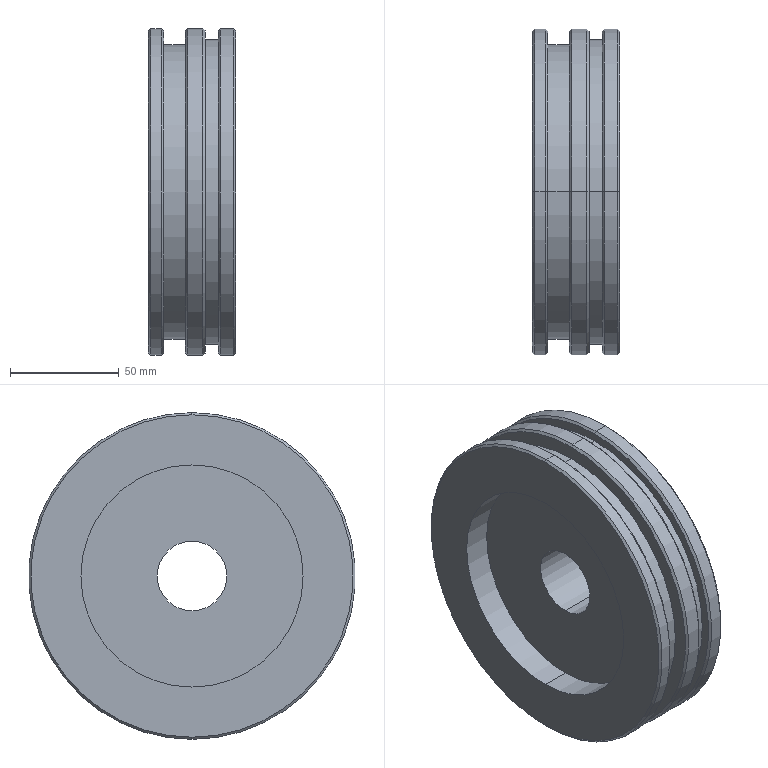Part | SolidWorks | features Chamfer 1, Revolution 1 | 1 solid | 39 faces | box 40 x 150 x 150 mm | volume 516029 mm3 | cone 16 | cylinder 14 | plane 9 | commonest cylinder face diameters 150 x6 32 x2 102 x2 135 x2 140 x2
STEP:
#1=CARTESIAN_POINT('',(0.,0.,74.));
#2=VERTEX_POINT('',#1);
#3=CARTESIAN_POINT('',(0.,0.,-74.));
#4=VERTEX_POINT('',#3);
#5=CARTESIAN_POINT('',(0.,0.,0.));
#6=DIRECTION('',(-1.,0.,0.));
#7=DIRECTION('',(0.,0.,-1.));
#8=AXIS2_PLACEMENT_3D('',#5,#6,#7);
#9=CIRCLE('',#8,74.);
#10=EDGE_CURVE('',#2,#4,#9,.T.);
#11=ORIENTED_EDGE('',*,*,#10,.F.);
#12=CARTESIAN_POINT('',(1.,0.,75.));
#13=VERTEX_POINT('',#12);
#14=CARTESIAN_POINT('',(0.,0.,74.));
#15=DIRECTION('',(0.7071,0.,0.7071));
#16=VECTOR('',#15,1000.);
#17=LINE('',#14,#16);
#18=EDGE_CURVE('',#2,#13,#17,.T.);
#19=ORIENTED_EDGE('',*,*,#18,.T.);
#20=CARTESIAN_POINT('',(1.,0.,-75.));
#21=VERTEX_POINT('',#20);
#22=CARTESIAN_POINT('',(1.,0.,0.));
#23=DIRECTION('',(1.,0.,0.));
#24=DIRECTION('',(0.,0.,-1.));
#25=AXIS2_PLACEMENT_3D('',#22,#23,#24);
#26=CIRCLE('',#25,75.);
#27=EDGE_CURVE('',#21,#13,#26,.T.);
#28=ORIENTED_EDGE('',*,*,#27,.F.);
#29=CARTESIAN_POINT('',(0.,0.,-74.));
#30=DIRECTION('',(0.7071,0.,-0.7071));
#31=VECTOR('',#30,1000.);
#32=LINE('',#29,#31);
#33=EDGE_CURVE('',#4,#21,#32,.T.);
#34=ORIENTED_EDGE('',*,*,#33,.F.);
#35=EDGE_LOOP('',(#11,#19,#28,#34));
#36=FACE_OUTER_BOUND('',#35,.T.);
#37=CARTESIAN_POINT('',(0.,0.,0.));
#38=DIRECTION('',(1.,0.,0.));
#39=DIRECTION('',(0.,0.,-1.));
#40=AXIS2_PLACEMENT_3D('',#37,#38,#39);
#41=CONICAL_SURFACE('',#40,74.,0.7854);
#42=ADVANCED_FACE('',(#36),#41,.T.);
#43=CARTESIAN_POINT('',(7.,0.,-74.));
#44=VERTEX_POINT('',#43);
#45=CARTESIAN_POINT('',(7.,0.,74.));
#46=VERTEX_POINT('',#45);
#47=CARTESIAN_POINT('',(7.,0.,0.));
#48=DIRECTION('',(1.,0.,0.));
#49=DIRECTION('',(0.,0.,1.));
#50=AXIS2_PLACEMENT_3D('',#47,#48,#49);
#51=CIRCLE('',#50,74.);
#52=EDGE_CURVE('',#44,#46,#51,.T.);
#53=ORIENTED_EDGE('',*,*,#52,.F.);
#54=CARTESIAN_POINT('',(6.,0.,-75.));
#55=VERTEX_POINT('',#54);
#56=CARTESIAN_POINT('',(6.,0.,-75.));
#57=DIRECTION('',(-0.7071,0.,-0.7071));
#58=VECTOR('',#57,1000.);
#59=LINE('',#56,#58);
#60=EDGE_CURVE('',#44,#55,#59,.T.);
#61=ORIENTED_EDGE('',*,*,#60,.T.);
#62=CARTESIAN_POINT('',(6.,0.,75.));
#63=VERTEX_POINT('',#62);
#64=CARTESIAN_POINT('',(6.,0.,0.));
#65=DIRECTION('',(-1.,0.,0.));
#66=DIRECTION('',(0.,0.,1.));
#67=AXIS2_PLACEMENT_3D('',#64,#65,#66);
#68=CIRCLE('',#67,75.);
#69=EDGE_CURVE('',#63,#55,#68,.T.);
#70=ORIENTED_EDGE('',*,*,#69,.F.);
#71=CARTESIAN_POINT('',(6.,0.,75.));
#72=DIRECTION('',(-0.7071,0.,0.7071));
#73=VECTOR('',#72,1000.);
#74=LINE('',#71,#73);
#75=EDGE_CURVE('',#46,#63,#74,.T.);
#76=ORIENTED_EDGE('',*,*,#75,.F.);
#77=EDGE_LOOP('',(#53,#61,#70,#76));
#78=FACE_OUTER_BOUND('',#77,.T.);
#79=CARTESIAN_POINT('',(6.,0.,0.));
#80=DIRECTION('',(-1.,0.,0.));
#81=DIRECTION('',(0.,0.,1.));
#82=AXIS2_PLACEMENT_3D('',#79,#80,#81);
#83=CONICAL_SURFACE('',#82,75.,0.7854);
#84=ADVANCED_FACE('',(#78),#83,.T.);
#85=CARTESIAN_POINT('',(17.,0.,74.));
#86=VERTEX_POINT('',#85);
#87=CARTESIAN_POINT('',(17.,0.,-74.));
#88=VERTEX_POINT('',#87);
#89=CARTESIAN_POINT('',(17.,0.,0.));
#90=DIRECTION('',(-1.,0.,0.));
#91=DIRECTION('',(0.,0.,-1.));
#92=AXIS2_PLACEMENT_3D('',#89,#90,#91);
#93=CIRCLE('',#92,74.);
#94=EDGE_CURVE('',#86,#88,#93,.T.);
#95=ORIENTED_EDGE('',*,*,#94,.F.);
#96=CARTESIAN_POINT('',(18.,0.,75.));
#97=VERTEX_POINT('',#96);
#98=CARTESIAN_POINT('',(17.,0.,74.));
#99=DIRECTION('',(0.7071,0.,0.7071));
#100=VECTOR('',#99,1000.);
#101=LINE('',#98,#100);
#102=EDGE_CURVE('',#86,#97,#101,.T.);
#103=ORIENTED_EDGE('',*,*,#102,.T.);
#104=CARTESIAN_POINT('',(18.,0.,-75.));
#105=VERTEX_POINT('',#104);
#106=CARTESIAN_POINT('',(18.,0.,0.));
#107=DIRECTION('',(1.,0.,0.));
#108=DIRECTION('',(0.,0.,-1.));
#109=AXIS2_PLACEMENT_3D('',#106,#107,#108);
#110=CIRCLE('',#109,75.);
#111=EDGE_CURVE('',#105,#97,#110,.T.);
#112=ORIENTED_EDGE('',*,*,#111,.F.);
#113=CARTESIAN_POINT('',(17.,0.,-74.));
#114=DIRECTION('',(0.7071,0.,-0.7071));
#115=VECTOR('',#114,1000.);
#116=LINE('',#113,#115);
#117=EDGE_CURVE('',#88,#105,#116,.T.);
#118=ORIENTED_EDGE('',*,*,#117,.F.);
#119=EDGE_LOOP('',(#95,#103,#112,#118));
#120=FACE_OUTER_BOUND('',#119,.T.);
#121=CARTESIAN_POINT('',(17.,0.,0.));
#122=DIRECTION('',(1.,0.,0.));
#123=DIRECTION('',(0.,0.,-1.));
#124=AXIS2_PLACEMENT_3D('',#121,#122,#123);
#125=CONICAL_SURFACE('',#124,74.,0.7854);
#126=ADVANCED_FACE('',(#120),#125,.T.);
#127=CARTESIAN_POINT('',(26.,0.,-74.));
#128=VERTEX_POINT('',#127);
#129=CARTESIAN_POINT('',(26.,0.,74.));
#130=VERTEX_POINT('',#129);
#131=CARTESIAN_POINT('',(26.,0.,0.));
#132=DIRECTION('',(1.,0.,0.));
#133=DIRECTION('',(0.,0.,1.));
#134=AXIS2_PLACEMENT_3D('',#131,#132,#133);
#135=CIRCLE('',#134,74.);
#136=EDGE_CURVE('',#128,#130,#135,.T.);
#137=ORIENTED_EDGE('',*,*,#136,.F.);
#138=CARTESIAN_POINT('',(25.,0.,-75.));
#139=VERTEX_POINT('',#138);
#140=CARTESIAN_POINT('',(25.,0.,-75.));
#141=DIRECTION('',(-0.7071,0.,-0.7071));
#142=VECTOR('',#141,1000.);
#143=LINE('',#140,#142);
#144=EDGE_CURVE('',#128,#139,#143,.T.);
#145=ORIENTED_EDGE('',*,*,#144,.T.);
#146=CARTESIAN_POINT('',(25.,0.,75.));
#147=VERTEX_POINT('',#146);
#148=CARTESIAN_POINT('',(25.,0.,0.));
#149=DIRECTION('',(-1.,0.,0.));
#150=DIRECTION('',(0.,0.,1.));
#151=AXIS2_PLACEMENT_3D('',#148,#149,#150);
#152=CIRCLE('',#151,75.);
#153=EDGE_CURVE('',#147,#139,#152,.T.);
#154=ORIENTED_EDGE('',*,*,#153,.F.);
#155=CARTESIAN_POINT('',(25.,0.,75.));
#156=DIRECTION('',(-0.7071,0.,0.7071));
#157=VECTOR('',#156,1000.);
#158=LINE('',#155,#157);
#159=EDGE_CURVE('',#130,#147,#158,.T.);
#160=ORIENTED_EDGE('',*,*,#159,.F.);
#161=EDGE_LOOP('',(#137,#145,#154,#160));
#162=FACE_OUTER_BOUND('',#161,.T.);
#163=CARTESIAN_POINT('',(25.,0.,0.));
#164=DIRECTION('',(-1.,0.,0.));
#165=DIRECTION('',(0.,0.,1.));
#166=AXIS2_PLACEMENT_3D('',#163,#164,#165);
#167=CONICAL_SURFACE('',#166,75.,0.7854);
#168=ADVANCED_FACE('',(#162),#167,.T.);
#169=CARTESIAN_POINT('',(32.,0.,74.));
#170=VERTEX_POINT('',#169);
#171=CARTESIAN_POINT('',(32.,0.,-74.));
#172=VERTEX_POINT('',#171);
#173=CARTESIAN_POINT('',(32.,0.,0.));
#174=DIRECTION('',(-1.,0.,0.));
#175=DIRECTION('',(0.,0.,-1.));
#176=AXIS2_PLACEMENT_3D('',#173,#174,#175);
#177=CIRCLE('',#176,74.);
#178=EDGE_CURVE('',#170,#172,#177,.T.);
#179=ORIENTED_EDGE('',*,*,#178,.F.);
#180=CARTESIAN_POINT('',(33.,0.,75.));
#181=VERTEX_POINT('',#180);
#182=CARTESIAN_POINT('',(32.,0.,74.));
#183=DIRECTION('',(0.7071,0.,0.7071));
#184=VECTOR('',#183,1000.);
#185=LINE('',#182,#184);
#186=EDGE_CURVE('',#170,#181,#185,.T.);
#187=ORIENTED_EDGE('',*,*,#186,.T.);
#188=CARTESIAN_POINT('',(33.,0.,-75.));
#189=VERTEX_POINT('',#188);
#190=CARTESIAN_POINT('',(33.,0.,0.));
#191=DIRECTION('',(1.,0.,0.));
#192=DIRECTION('',(0.,0.,-1.));
#193=AXIS2_PLACEMENT_3D('',#190,#191,#192);
#194=CIRCLE('',#193,75.);
#195=EDGE_CURVE('',#189,#181,#194,.T.);
#196=ORIENTED_EDGE('',*,*,#195,.F.);
#197=CARTESIAN_POINT('',(32.,0.,-74.));
#198=DIRECTION('',(0.7071,0.,-0.7071));
#199=VECTOR('',#198,1000.);
#200=LINE('',#197,#199);
#201=EDGE_CURVE('',#172,#189,#200,.T.);
#202=ORIENTED_EDGE('',*,*,#201,.F.);
#203=EDGE_LOOP('',(#179,#187,#196,#202));
#204=FACE_OUTER_BOUND('',#203,.T.);
#205=CARTESIAN_POINT('',(32.,0.,0.));
#206=DIRECTION('',(1.,0.,0.));
#207=DIRECTION('',(0.,0.,-1.));
#208=AXIS2_PLACEMENT_3D('',#205,#206,#207);
#209=CONICAL_SURFACE('',#208,74.,0.7854);
#210=ADVANCED_FACE('',(#204),#209,.T.);
#211=CARTESIAN_POINT('',(40.,0.,-74.));
#212=VERTEX_POINT('',#211);
#213=CARTESIAN_POINT('',(40.,0.,74.));
#214=VERTEX_POINT('',#213);
#215=CARTESIAN_POINT('',(40.,0.,0.));
#216=DIRECTION('',(1.,0.,0.));
#217=DIRECTION('',(0.,0.,1.));
#218=AXIS2_PLACEMENT_3D('',#215,#216,#217);
#219=CIRCLE('',#218,74.);
#220=EDGE_CURVE('',#212,#214,#219,.T.);
#221=ORIENTED_EDGE('',*,*,#220,.F.);
#222=CARTESIAN_POINT('',(39.,0.,-75.));
#223=VERTEX_POINT('',#222);
#224=CARTESIAN_POINT('',(39.,0.,-75.));
#225=DIRECTION('',(-0.7071,0.,-0.7071));
#226=VECTOR('',#225,1000.);
#227=LINE('',#224,#226);
#228=EDGE_CURVE('',#212,#223,#227,.T.);
#229=ORIENTED_EDGE('',*,*,#228,.T.);
#230=CARTESIAN_POINT('',(39.,0.,75.));
#231=VERTEX_POINT('',#230);
#232=CARTESIAN_POINT('',(39.,0.,0.));
#233=DIRECTION('',(-1.,0.,0.));
#234=DIRECTION('',(0.,0.,1.));
#235=AXIS2_PLACEMENT_3D('',#232,#233,#234);
#236=CIRCLE('',#235,75.);
#237=EDGE_CURVE('',#231,#223,#236,.T.);
#238=ORIENTED_EDGE('',*,*,#237,.F.);
#239=CARTESIAN_POINT('',(39.,0.,75.));
#240=DIRECTION('',(-0.7071,0.,0.7071));
#241=VECTOR('',#240,1000.);
#242=LINE('',#239,#241);
#243=EDGE_CURVE('',#214,#231,#242,.T.);
#244=ORIENTED_EDGE('',*,*,#243,.F.);
#245=EDGE_LOOP('',(#221,#229,#238,#244));
#246=FACE_OUTER_BOUND('',#245,.T.);
#247=CARTESIAN_POINT('',(39.,0.,0.));
#248=DIRECTION('',(-1.,0.,0.));
#249=DIRECTION('',(0.,0.,1.));
#250=AXIS2_PLACEMENT_3D('',#247,#248,#249);
#251=CONICAL_SURFACE('',#250,75.,0.7854);
#252=ADVANCED_FACE('',(#246),#251,.T.);
#253=CARTESIAN_POINT('',(40.,0.,-16.));
#254=VERTEX_POINT('',#253);
#255=CARTESIAN_POINT('',(40.,0.,16.));
#256=VERTEX_POINT('',#255);
#257=CARTESIAN_POINT('',(40.,0.,0.));
#258=DIRECTION('',(-1.,0.,0.));
#259=DIRECTION('',(0.,0.,1.));
#260=AXIS2_PLACEMENT_3D('',#257,#258,#259);
#261=CIRCLE('',#260,16.);
#262=EDGE_CURVE('',#254,#256,#261,.T.);
#263=ORIENTED_EDGE('',*,*,#262,.F.);
#264=CARTESIAN_POINT('',(13.,0.,-16.));
#265=VERTEX_POINT('',#264);
#266=CARTESIAN_POINT('',(0.,0.,-16.));
#267=DIRECTION('',(-1.,0.,0.));
#268=VECTOR('',#267,1000.);
#269=LINE('',#266,#268);
#270=EDGE_CURVE('',#254,#265,#269,.T.);
#271=ORIENTED_EDGE('',*,*,#270,.T.);
#272=CARTESIAN_POINT('',(13.,0.,16.));
#273=VERTEX_POINT('',#272);
#274=CARTESIAN_POINT('',(13.,0.,0.));
#275=DIRECTION('',(-1.,0.,0.));
#276=DIRECTION('',(0.,0.,1.));
#277=AXIS2_PLACEMENT_3D('',#274,#275,#276);
#278=CIRCLE('',#277,16.);
#279=EDGE_CURVE('',#265,#273,#278,.T.);
#280=ORIENTED_EDGE('',*,*,#279,.T.);
#281=CARTESIAN_POINT('',(0.,0.,16.));
#282=DIRECTION('',(-1.,0.,0.));
#283=VECTOR('',#282,1000.);
#284=LINE('',#281,#283);
#285=EDGE_CURVE('',#256,#273,#284,.T.);
#286=ORIENTED_EDGE('',*,*,#285,.F.);
#287=EDGE_LOOP('',(#263,#271,#280,#286));
#288=FACE_OUTER_BOUND('',#287,.T.);
#289=CARTESIAN_POINT('',(0.,0.,0.));
#290=DIRECTION('',(-1.,0.,0.));
#291=DIRECTION('',(0.,0.,1.));
#292=AXIS2_PLACEMENT_3D('',#289,#290,#291);
#293=CYLINDRICAL_SURFACE('',#292,16.);
#294=ADVANCED_FACE('',(#288),#293,.F.);
#295=CARTESIAN_POINT('',(40.,0.,33.));
#296=VERTEX_POINT('',#295);
#297=CARTESIAN_POINT('',(40.,0.,-33.));
#298=VERTEX_POINT('',#297);
#299=CARTESIAN_POINT('',(40.,0.,0.));
#300=DIRECTION('',(-1.,0.,0.));
#301=DIRECTION('',(0.,0.,1.));
#302=AXIS2_PLACEMENT_3D('',#299,#300,#301);
#303=CIRCLE('',#302,33.);
#304=EDGE_CURVE('',#296,#298,#303,.T.);
#305=ORIENTED_EDGE('',*,*,#304,.T.);
#306=CARTESIAN_POINT('',(38.,0.,-35.));
#307=VERTEX_POINT('',#306);
#308=CARTESIAN_POINT('',(40.,0.,-33.));
#309=DIRECTION('',(-0.7071,0.,-0.7071));
#310=VECTOR('',#309,1000.);
#311=LINE('',#308,#310);
#312=EDGE_CURVE('',#298,#307,#311,.T.);
#313=ORIENTED_EDGE('',*,*,#312,.T.);
#314=CARTESIAN_POINT('',(38.,0.,35.));
#315=VERTEX_POINT('',#314);
#316=CARTESIAN_POINT('',(38.,0.,0.));
#317=DIRECTION('',(-1.,0.,0.));
#318=DIRECTION('',(0.,0.,1.));
#319=AXIS2_PLACEMENT_3D('',#316,#317,#318);
#320=CIRCLE('',#319,35.);
#321=EDGE_CURVE('',#315,#307,#320,.T.);
#322=ORIENTED_EDGE('',*,*,#321,.F.);
#323=CARTESIAN_POINT('',(40.,0.,33.));
#324=DIRECTION('',(-0.7071,0.,0.7071));
#325=VECTOR('',#324,1000.);
#326=LINE('',#323,#325);
#327=EDGE_CURVE('',#296,#315,#326,.T.);
#328=ORIENTED_EDGE('',*,*,#327,.F.);
#329=EDGE_LOOP('',(#305,#313,#322,#328));
#330=FACE_OUTER_BOUND('',#329,.T.);
#331=CARTESIAN_POINT('',(40.,0.,0.));
#332=DIRECTION('',(-1.,0.,0.));
#333=DIRECTION('',(0.,0.,1.));
#334=AXIS2_PLACEMENT_3D('',#331,#332,#333);
#335=CONICAL_SURFACE('',#334,33.,0.7854);
#336=ADVANCED_FACE('',(#330),#335,.T.);
#337=CARTESIAN_POINT('',(38.,0.,-57.5));
#338=VERTEX_POINT('',#337);
#339=CARTESIAN_POINT('',(38.,0.,57.5));
#340=VERTEX_POINT('',#339);
#341=CARTESIAN_POINT('',(38.,0.,0.));
#342=DIRECTION('',(-1.,0.,0.));
#343=DIRECTION('',(0.,0.,1.));
#344=AXIS2_PLACEMENT_3D('',#341,#342,#343);
#345=CIRCLE('',#344,57.5);
#346=EDGE_CURVE('',#338,#340,#345,.T.);
#347=ORIENTED_EDGE('',*,*,#346,.T.);
#348=CARTESIAN_POINT('',(40.,0.,59.5));
#349=VERTEX_POINT('',#348);
#350=CARTESIAN_POINT('',(38.,0.,57.5));
#351=DIRECTION('',(0.7071,0.,0.7071));
#352=VECTOR('',#351,1000.);
#353=LINE('',#350,#352);
#354=EDGE_CURVE('',#340,#349,#353,.T.);
#355=ORIENTED_EDGE('',*,*,#354,.T.);
#356=CARTESIAN_POINT('',(40.,0.,-59.5));
#357=VERTEX_POINT('',#356);
#358=CARTESIAN_POINT('',(40.,0.,0.));
#359=DIRECTION('',(-1.,0.,0.));
#360=DIRECTION('',(0.,0.,1.));
#361=AXIS2_PLACEMENT_3D('',#358,#359,#360);
#362=CIRCLE('',#361,59.5);
#363=EDGE_CURVE('',#357,#349,#362,.T.);
#364=ORIENTED_EDGE('',*,*,#363,.F.);
#365=CARTESIAN_POINT('',(38.,0.,-57.5));
#366=DIRECTION('',(0.7071,0.,-0.7071));
#367=VECTOR('',#366,1000.);
#368=LINE('',#365,#367);
#369=EDGE_CURVE('',#338,#357,#368,.T.);
#370=ORIENTED_EDGE('',*,*,#369,.F.);
#371=EDGE_LOOP('',(#347,#355,#364,#370));
#372=FACE_OUTER_BOUND('',#371,.T.);
#373=CARTESIAN_POINT('',(38.,0.,0.));
#374=DIRECTION('',(1.,0.,0.));
#375=DIRECTION('',(0.,0.,-1.));
#376=AXIS2_PLACEMENT_3D('',#373,#374,#375);
#377=CONICAL_SURFACE('',#376,57.5,0.7854);
#378=ADVANCED_FACE('',(#372),#377,.F.);
#379=ORIENTED_EDGE('',*,*,#237,.T.);
#380=CARTESIAN_POINT('',(0.,0.,-75.));
#381=DIRECTION('',(-1.,0.,0.));
#382=VECTOR('',#381,1000.);
#383=LINE('',#380,#382);
#384=EDGE_CURVE('',#223,#189,#383,.T.);
#385=ORIENTED_EDGE('',*,*,#384,.T.);
#386=ORIENTED_EDGE('',*,*,#195,.T.);
#387=CARTESIAN_POINT('',(0.,0.,75.));
#388=DIRECTION('',(-1.,0.,0.));
#389=VECTOR('',#388,1000.);
#390=LINE('',#387,#389);
#391=EDGE_CURVE('',#231,#181,#390,.T.);
#392=ORIENTED_EDGE('',*,*,#391,.F.);
#393=EDGE_LOOP('',(#379,#385,#386,#392));
#394=FACE_OUTER_BOUND('',#393,.T.);
#395=CARTESIAN_POINT('',(0.,0.,0.));
#396=DIRECTION('',(-1.,0.,0.));
#397=DIRECTION('',(0.,0.,1.));
#398=AXIS2_PLACEMENT_3D('',#395,#396,#397);
#399=CYLINDRICAL_SURFACE('',#398,75.);
#400=ADVANCED_FACE('',(#394),#399,.T.);
#401=CARTESIAN_POINT('',(32.,0.,70.));
#402=VERTEX_POINT('',#401);
#403=CARTESIAN_POINT('',(32.,0.,-70.));
#404=VERTEX_POINT('',#403);
#405=CARTESIAN_POINT('',(32.,0.,0.));
#406=DIRECTION('',(-1.,0.,0.));
#407=DIRECTION('',(0.,0.,1.));
#408=AXIS2_PLACEMENT_3D('',#405,#406,#407);
#409=CIRCLE('',#408,70.);
#410=EDGE_CURVE('',#402,#404,#409,.T.);
#411=ORIENTED_EDGE('',*,*,#410,.T.);
#412=CARTESIAN_POINT('',(26.,0.,-70.));
#413=VERTEX_POINT('',#412);
#414=CARTESIAN_POINT('',(0.,0.,-70.));
#415=DIRECTION('',(-1.,0.,0.));
#416=VECTOR('',#415,1000.);
#417=LINE('',#414,#416);
#418=EDGE_CURVE('',#404,#413,#417,.T.);
#419=ORIENTED_EDGE('',*,*,#418,.T.);
#420=CARTESIAN_POINT('',(26.,0.,70.));
#421=VERTEX_POINT('',#420);
#422=CARTESIAN_POINT('',(26.,0.,0.));
#423=DIRECTION('',(-1.,0.,0.));
#424=DIRECTION('',(0.,0.,1.));
#425=AXIS2_PLACEMENT_3D('',#422,#423,#424);
#426=CIRCLE('',#425,70.);
#427=EDGE_CURVE('',#421,#413,#426,.T.);
#428=ORIENTED_EDGE('',*,*,#427,.F.);
#429=CARTESIAN_POINT('',(0.,0.,70.));
#430=DIRECTION('',(-1.,0.,0.));
#431=VECTOR('',#430,1000.);
#432=LINE('',#429,#431);
#433=EDGE_CURVE('',#402,#421,#432,.T.);
#434=ORIENTED_EDGE('',*,*,#433,.F.);
#435=EDGE_LOOP('',(#411,#419,#428,#434));
#436=FACE_OUTER_BOUND('',#435,.T.);
#437=CARTESIAN_POINT('',(0.,0.,0.));
#438=DIRECTION('',(-1.,0.,0.));
#439=DIRECTION('',(0.,0.,1.));
#440=AXIS2_PLACEMENT_3D('',#437,#438,#439);
#441=CYLINDRICAL_SURFACE('',#440,70.);
#442=ADVANCED_FACE('',(#436),#441,.T.);
#443=ORIENTED_EDGE('',*,*,#153,.T.);
#444=CARTESIAN_POINT('',(0.,0.,-75.));
#445=DIRECTION('',(-1.,0.,0.));
#446=VECTOR('',#445,1000.);
#447=LINE('',#444,#446);
#448=EDGE_CURVE('',#139,#105,#447,.T.);
#449=ORIENTED_EDGE('',*,*,#448,.T.);
#450=ORIENTED_EDGE('',*,*,#111,.T.);
#451=CARTESIAN_POINT('',(0.,0.,75.));
#452=DIRECTION('',(-1.,0.,0.));
#453=VECTOR('',#452,1000.);
#454=LINE('',#451,#453);
#455=EDGE_CURVE('',#147,#97,#454,.T.);
#456=ORIENTED_EDGE('',*,*,#455,.F.);
#457=EDGE_LOOP('',(#443,#449,#450,#456));
#458=FACE_OUTER_BOUND('',#457,.T.);
#459=CARTESIAN_POINT('',(0.,0.,0.));
#460=DIRECTION('',(-1.,0.,0.));
#461=DIRECTION('',(0.,0.,1.));
#462=AXIS2_PLACEMENT_3D('',#459,#460,#461);
#463=CYLINDRICAL_SURFACE('',#462,75.);
#464=ADVANCED_FACE('',(#458),#463,.T.);
#465=CARTESIAN_POINT('',(17.,0.,67.5));
#466=VERTEX_POINT('',#465);
#467=CARTESIAN_POINT('',(17.,0.,-67.5));
#468=VERTEX_POINT('',#467);
#469=CARTESIAN_POINT('',(17.,0.,0.));
#470=DIRECTION('',(-1.,0.,0.));
#471=DIRECTION('',(0.,0.,1.));
#472=AXIS2_PLACEMENT_3D('',#469,#470,#471);
#473=CIRCLE('',#472,67.5);
#474=EDGE_CURVE('',#466,#468,#473,.T.);
#475=ORIENTED_EDGE('',*,*,#474,.T.);
#476=CARTESIAN_POINT('',(7.,0.,-67.5));
#477=VERTEX_POINT('',#476);
#478=CARTESIAN_POINT('',(0.,0.,-67.5));
#479=DIRECTION('',(-1.,0.,0.));
#480=VECTOR('',#479,1000.);
#481=LINE('',#478,#480);
#482=EDGE_CURVE('',#468,#477,#481,.T.);
#483=ORIENTED_EDGE('',*,*,#482,.T.);
#484=CARTESIAN_POINT('',(7.,0.,67.5));
#485=VERTEX_POINT('',#484);
#486=CARTESIAN_POINT('',(7.,0.,0.));
#487=DIRECTION('',(-1.,0.,0.));
#488=DIRECTION('',(0.,0.,1.));
#489=AXIS2_PLACEMENT_3D('',#486,#487,#488);
#490=CIRCLE('',#489,67.5);
#491=EDGE_CURVE('',#485,#477,#490,.T.);
#492=ORIENTED_EDGE('',*,*,#491,.F.);
#493=CARTESIAN_POINT('',(0.,0.,67.5));
#494=DIRECTION('',(-1.,0.,0.));
#495=VECTOR('',#494,1000.);
#496=LINE('',#493,#495);
#497=EDGE_CURVE('',#466,#485,#496,.T.);
#498=ORIENTED_EDGE('',*,*,#497,.F.);
#499=EDGE_LOOP('',(#475,#483,#492,#498));
#500=FACE_OUTER_BOUND('',#499,.T.);
#501=CARTESIAN_POINT('',(0.,0.,0.));
#502=DIRECTION('',(-1.,0.,0.));
#503=DIRECTION('',(0.,0.,1.));
#504=AXIS2_PLACEMENT_3D('',#501,#502,#503);
#505=CYLINDRICAL_SURFACE('',#504,67.5);
#506=ADVANCED_FACE('',(#500),#505,.T.);
#507=ORIENTED_EDGE('',*,*,#69,.T.);
#508=CARTESIAN_POINT('',(0.,0.,-75.));
#509=DIRECTION('',(-1.,0.,0.));
#510=VECTOR('',#509,1000.);
#511=LINE('',#508,#510);
#512=EDGE_CURVE('',#55,#21,#511,.T.);
#513=ORIENTED_EDGE('',*,*,#512,.T.);
#514=ORIENTED_EDGE('',*,*,#27,.T.);
#515=CARTESIAN_POINT('',(0.,0.,75.));
#516=DIRECTION('',(-1.,0.,0.));
#517=VECTOR('',#516,1000.);
#518=LINE('',#515,#517);
#519=EDGE_CURVE('',#63,#13,#518,.T.);
#520=ORIENTED_EDGE('',*,*,#519,.F.);
#521=EDGE_LOOP('',(#507,#513,#514,#520));
#522=FACE_OUTER_BOUND('',#521,.T.);
#523=CARTESIAN_POINT('',(0.,0.,0.));
#524=DIRECTION('',(-1.,0.,0.));
#525=DIRECTION('',(0.,0.,1.));
#526=AXIS2_PLACEMENT_3D('',#523,#524,#525);
#527=CYLINDRICAL_SURFACE('',#526,75.);
#528=ADVANCED_FACE('',(#522),#527,.T.);
#529=CARTESIAN_POINT('',(13.,0.,-51.));
#530=VERTEX_POINT('',#529);
#531=CARTESIAN_POINT('',(13.,0.,51.));
#532=VERTEX_POINT('',#531);
#533=CARTESIAN_POINT('',(13.,0.,0.));
#534=DIRECTION('',(-1.,0.,0.));
#535=DIRECTION('',(0.,0.,1.));
#536=AXIS2_PLACEMENT_3D('',#533,#534,#535);
#537=CIRCLE('',#536,51.);
#538=EDGE_CURVE('',#530,#532,#537,.T.);
#539=ORIENTED_EDGE('',*,*,#538,.F.);
#540=CARTESIAN_POINT('',(0.,0.,-51.));
#541=VERTEX_POINT('',#540);
#542=CARTESIAN_POINT('',(0.,0.,-51.));
#543=DIRECTION('',(-1.,0.,0.));
#544=VECTOR('',#543,1000.);
#545=LINE('',#542,#544);
#546=EDGE_CURVE('',#530,#541,#545,.T.);
#547=ORIENTED_EDGE('',*,*,#546,.T.);
#548=CARTESIAN_POINT('',(0.,0.,51.));
#549=VERTEX_POINT('',#548);
#550=CARTESIAN_POINT('',(0.,0.,0.));
#551=DIRECTION('',(-1.,0.,0.));
#552=DIRECTION('',(0.,0.,1.));
#553=AXIS2_PLACEMENT_3D('',#550,#551,#552);
#554=CIRCLE('',#553,51.);
#555=EDGE_CURVE('',#541,#549,#554,.T.);
#556=ORIENTED_EDGE('',*,*,#555,.T.);
#557=CARTESIAN_POINT('',(0.,0.,51.));
#558=DIRECTION('',(-1.,0.,0.));
#559=VECTOR('',#558,1000.);
#560=LINE('',#557,#559);
#561=EDGE_CURVE('',#532,#549,#560,.T.);
#562=ORIENTED_EDGE('',*,*,#561,.F.);
#563=EDGE_LOOP('',(#539,#547,#556,#562));
#564=FACE_OUTER_BOUND('',#563,.T.);
#565=CARTESIAN_POINT('',(0.,0.,0.));
#566=DIRECTION('',(-1.,0.,0.));
#567=DIRECTION('',(0.,0.,1.));
#568=AXIS2_PLACEMENT_3D('',#565,#566,#567);
#569=CYLINDRICAL_SURFACE('',#568,51.);
#570=ADVANCED_FACE('',(#564),#569,.F.);
#571=ORIENTED_EDGE('',*,*,#546,.F.);
#572=CARTESIAN_POINT('',(13.,0.,0.));
#573=DIRECTION('',(-1.,0.,0.));
#574=DIRECTION('',(0.,0.,1.));
#575=AXIS2_PLACEMENT_3D('',#572,#573,#574);
#576=CIRCLE('',#575,51.);
#577=EDGE_CURVE('',#532,#530,#576,.T.);
#578=ORIENTED_EDGE('',*,*,#577,.F.);
#579=ORIENTED_EDGE('',*,*,#561,.T.);
#580=CARTESIAN_POINT('',(0.,0.,0.));
#581=DIRECTION('',(-1.,0.,0.));
#582=DIRECTION('',(0.,0.,1.));
#583=AXIS2_PLACEMENT_3D('',#580,#581,#582);
#584=CIRCLE('',#583,51.);
#585=EDGE_CURVE('',#549,#541,#584,.T.);
#586=ORIENTED_EDGE('',*,*,#585,.T.);
#587=EDGE_LOOP('',(#571,#578,#579,#586));
#588=FACE_OUTER_BOUND('',#587,.T.);
#589=CARTESIAN_POINT('',(0.,0.,0.));
#590=DIRECTION('',(-1.,0.,0.));
#591=DIRECTION('',(0.,0.,1.));
#592=AXIS2_PLACEMENT_3D('',#589,#590,#591);
#593=CYLINDRICAL_SURFACE('',#592,51.);
#594=ADVANCED_FACE('',(#588),#593,.F.);
#595=CARTESIAN_POINT('',(0.,0.,0.));
#596=DIRECTION('',(-1.,0.,0.));
#597=DIRECTION('',(0.,0.,-1.));
#598=AXIS2_PLACEMENT_3D('',#595,#596,#597);
#599=CIRCLE('',#598,74.);
#600=EDGE_CURVE('',#4,#2,#599,.T.);
#601=ORIENTED_EDGE('',*,*,#600,.T.);
#602=ORIENTED_EDGE('',*,*,#10,.T.);
#603=EDGE_LOOP('',(#601,#602));
#604=FACE_OUTER_BOUND('',#603,.T.);
#605=ORIENTED_EDGE('',*,*,#585,.F.);
#606=ORIENTED_EDGE('',*,*,#555,.F.);
#607=EDGE_LOOP('',(#605,#606));
#608=FACE_BOUND('',#607,.T.);
#609=CARTESIAN_POINT('',(0.,51.,0.));
#610=DIRECTION('',(1.,0.,0.));
#611=DIRECTION('',(0.,0.,-1.));
#612=AXIS2_PLACEMENT_3D('',#609,#610,#611);
#613=PLANE('',#612);
#614=ADVANCED_FACE('',(#604,#608),#613,.F.);
#615=ORIENTED_EDGE('',*,*,#512,.F.);
#616=CARTESIAN_POINT('',(6.,0.,0.));
#617=DIRECTION('',(-1.,0.,0.));
#618=DIRECTION('',(0.,0.,1.));
#619=AXIS2_PLACEMENT_3D('',#616,#617,#618);
#620=CIRCLE('',#619,75.);
#621=EDGE_CURVE('',#55,#63,#620,.T.);
#622=ORIENTED_EDGE('',*,*,#621,.T.);
#623=ORIENTED_EDGE('',*,*,#519,.T.);
#624=CARTESIAN_POINT('',(1.,0.,0.));
#625=DIRECTION('',(1.,0.,0.));
#626=DIRECTION('',(0.,0.,-1.));
#627=AXIS2_PLACEMENT_3D('',#624,#625,#626);
#628=CIRCLE('',#627,75.);
#629=EDGE_CURVE('',#13,#21,#628,.T.);
#630=ORIENTED_EDGE('',*,*,#629,.T.);
#631=EDGE_LOOP('',(#615,#622,#623,#630));
#632=FACE_OUTER_BOUND('',#631,.T.);
#633=CARTESIAN_POINT('',(0.,0.,0.));
#634=DIRECTION('',(-1.,0.,0.));
#635=DIRECTION('',(0.,0.,1.));
#636=AXIS2_PLACEMENT_3D('',#633,#634,#635);
#637=CYLINDRICAL_SURFACE('',#636,75.);
#638=ADVANCED_FACE('',(#632),#637,.T.);
#639=CARTESIAN_POINT('',(7.,0.,0.));
#640=DIRECTION('',(1.,0.,0.));
#641=DIRECTION('',(0.,0.,1.));
#642=AXIS2_PLACEMENT_3D('',#639,#640,#641);
#643=CIRCLE('',#642,74.);
#644=EDGE_CURVE('',#46,#44,#643,.T.);
#645=ORIENTED_EDGE('',*,*,#644,.T.);
#646=ORIENTED_EDGE('',*,*,#52,.T.);
#647=EDGE_LOOP('',(#645,#646));
#648=FACE_OUTER_BOUND('',#647,.T.);
#649=ORIENTED_EDGE('',*,*,#491,.T.);
#650=CARTESIAN_POINT('',(7.,0.,0.));
#651=DIRECTION('',(-1.,0.,0.));
#652=DIRECTION('',(0.,0.,1.));
#653=AXIS2_PLACEMENT_3D('',#650,#651,#652);
#654=CIRCLE('',#653,67.5);
#655=EDGE_CURVE('',#477,#485,#654,.T.);
#656=ORIENTED_EDGE('',*,*,#655,.T.);
#657=EDGE_LOOP('',(#649,#656));
#658=FACE_BOUND('',#657,.T.);
#659=CARTESIAN_POINT('',(7.,75.,0.));
#660=DIRECTION('',(-1.,0.,0.));
#661=DIRECTION('',(0.,0.,1.));
#662=AXIS2_PLACEMENT_3D('',#659,#660,#661);
#663=PLANE('',#662);
#664=ADVANCED_FACE('',(#648,#658),#663,.F.);
#665=ORIENTED_EDGE('',*,*,#482,.F.);
#666=CARTESIAN_POINT('',(17.,0.,0.));
#667=DIRECTION('',(-1.,0.,0.));
#668=DIRECTION('',(0.,0.,1.));
#669=AXIS2_PLACEMENT_3D('',#666,#667,#668);
#670=CIRCLE('',#669,67.5);
#671=EDGE_CURVE('',#468,#466,#670,.T.);
#672=ORIENTED_EDGE('',*,*,#671,.T.);
#673=ORIENTED_EDGE('',*,*,#497,.T.);
#674=ORIENTED_EDGE('',*,*,#655,.F.);
#675=EDGE_LOOP('',(#665,#672,#673,#674));
#676=FACE_OUTER_BOUND('',#675,.T.);
#677=CARTESIAN_POINT('',(0.,0.,0.));
#678=DIRECTION('',(-1.,0.,0.));
#679=DIRECTION('',(0.,0.,1.));
#680=AXIS2_PLACEMENT_3D('',#677,#678,#679);
#681=CYLINDRICAL_SURFACE('',#680,67.5);
#682=ADVANCED_FACE('',(#676),#681,.T.);
#683=CARTESIAN_POINT('',(17.,0.,0.));
#684=DIRECTION('',(-1.,0.,0.));
#685=DIRECTION('',(0.,0.,-1.));
#686=AXIS2_PLACEMENT_3D('',#683,#684,#685);
#687=CIRCLE('',#686,74.);
#688=EDGE_CURVE('',#88,#86,#687,.T.);
#689=ORIENTED_EDGE('',*,*,#688,.T.);
#690=ORIENTED_EDGE('',*,*,#94,.T.);
#691=EDGE_LOOP('',(#689,#690));
#692=FACE_OUTER_BOUND('',#691,.T.);
#693=ORIENTED_EDGE('',*,*,#474,.F.);
#694=ORIENTED_EDGE('',*,*,#671,.F.);
#695=EDGE_LOOP('',(#693,#694));
#696=FACE_BOUND('',#695,.T.);
#697=CARTESIAN_POINT('',(17.,67.5,0.));
#698=DIRECTION('',(1.,0.,0.));
#699=DIRECTION('',(0.,0.,-1.));
#700=AXIS2_PLACEMENT_3D('',#697,#698,#699);
#701=PLANE('',#700);
#702=ADVANCED_FACE('',(#692,#696),#701,.F.);
#703=ORIENTED_EDGE('',*,*,#448,.F.);
#704=CARTESIAN_POINT('',(25.,0.,0.));
#705=DIRECTION('',(-1.,0.,0.));
#706=DIRECTION('',(0.,0.,1.));
#707=AXIS2_PLACEMENT_3D('',#704,#705,#706);
#708=CIRCLE('',#707,75.);
#709=EDGE_CURVE('',#139,#147,#708,.T.);
#710=ORIENTED_EDGE('',*,*,#709,.T.);
#711=ORIENTED_EDGE('',*,*,#455,.T.);
#712=CARTESIAN_POINT('',(18.,0.,0.));
#713=DIRECTION('',(1.,0.,0.));
#714=DIRECTION('',(0.,0.,-1.));
#715=AXIS2_PLACEMENT_3D('',#712,#713,#714);
#716=CIRCLE('',#715,75.);
#717=EDGE_CURVE('',#97,#105,#716,.T.);
#718=ORIENTED_EDGE('',*,*,#717,.T.);
#719=EDGE_LOOP('',(#703,#710,#711,#718));
#720=FACE_OUTER_BOUND('',#719,.T.);
#721=CARTESIAN_POINT('',(0.,0.,0.));
#722=DIRECTION('',(-1.,0.,0.));
#723=DIRECTION('',(0.,0.,1.));
#724=AXIS2_PLACEMENT_3D('',#721,#722,#723);
#725=CYLINDRICAL_SURFACE('',#724,75.);
#726=ADVANCED_FACE('',(#720),#725,.T.);
#727=CARTESIAN_POINT('',(26.,0.,0.));
#728=DIRECTION('',(1.,0.,0.));
#729=DIRECTION('',(0.,0.,1.));
#730=AXIS2_PLACEMENT_3D('',#727,#728,#729);
#731=CIRCLE('',#730,74.);
#732=EDGE_CURVE('',#130,#128,#731,.T.);
#733=ORIENTED_EDGE('',*,*,#732,.T.);
#734=ORIENTED_EDGE('',*,*,#136,.T.);
#735=EDGE_LOOP('',(#733,#734));
#736=FACE_OUTER_BOUND('',#735,.T.);
#737=ORIENTED_EDGE('',*,*,#427,.T.);
#738=CARTESIAN_POINT('',(26.,0.,0.));
#739=DIRECTION('',(-1.,0.,0.));
#740=DIRECTION('',(0.,0.,1.));
#741=AXIS2_PLACEMENT_3D('',#738,#739,#740);
#742=CIRCLE('',#741,70.);
#743=EDGE_CURVE('',#413,#421,#742,.T.);
#744=ORIENTED_EDGE('',*,*,#743,.T.);
#745=EDGE_LOOP('',(#737,#744));
#746=FACE_BOUND('',#745,.T.);
#747=CARTESIAN_POINT('',(26.,75.,0.));
#748=DIRECTION('',(-1.,0.,0.));
#749=DIRECTION('',(0.,0.,1.));
#750=AXIS2_PLACEMENT_3D('',#747,#748,#749);
#751=PLANE('',#750);
#752=ADVANCED_FACE('',(#736,#746),#751,.F.);
#753=ORIENTED_EDGE('',*,*,#418,.F.);
#754=CARTESIAN_POINT('',(32.,0.,0.));
#755=DIRECTION('',(-1.,0.,0.));
#756=DIRECTION('',(0.,0.,1.));
#757=AXIS2_PLACEMENT_3D('',#754,#755,#756);
#758=CIRCLE('',#757,70.);
#759=EDGE_CURVE('',#404,#402,#758,.T.);
#760=ORIENTED_EDGE('',*,*,#759,.T.);
#761=ORIENTED_EDGE('',*,*,#433,.T.);
#762=ORIENTED_EDGE('',*,*,#743,.F.);
#763=EDGE_LOOP('',(#753,#760,#761,#762));
#764=FACE_OUTER_BOUND('',#763,.T.);
#765=CARTESIAN_POINT('',(0.,0.,0.));
#766=DIRECTION('',(-1.,0.,0.));
#767=DIRECTION('',(0.,0.,1.));
#768=AXIS2_PLACEMENT_3D('',#765,#766,#767);
#769=CYLINDRICAL_SURFACE('',#768,70.);
#770=ADVANCED_FACE('',(#764),#769,.T.);
#771=CARTESIAN_POINT('',(32.,0.,0.));
#772=DIRECTION('',(-1.,0.,0.));
#773=DIRECTION('',(0.,0.,-1.));
#774=AXIS2_PLACEMENT_3D('',#771,#772,#773);
#775=CIRCLE('',#774,74.);
#776=EDGE_CURVE('',#172,#170,#775,.T.);
#777=ORIENTED_EDGE('',*,*,#776,.T.);
#778=ORIENTED_EDGE('',*,*,#178,.T.);
#779=EDGE_LOOP('',(#777,#778));
#780=FACE_OUTER_BOUND('',#779,.T.);
#781=ORIENTED_EDGE('',*,*,#410,.F.);
#782=ORIENTED_EDGE('',*,*,#759,.F.);
#783=EDGE_LOOP('',(#781,#782));
#784=FACE_BOUND('',#783,.T.);
#785=CARTESIAN_POINT('',(32.,70.,0.));
#786=DIRECTION('',(1.,0.,0.));
#787=DIRECTION('',(0.,0.,-1.));
#788=AXIS2_PLACEMENT_3D('',#785,#786,#787);
#789=PLANE('',#788);
#790=ADVANCED_FACE('',(#780,#784),#789,.F.);
#791=ORIENTED_EDGE('',*,*,#384,.F.);
#792=CARTESIAN_POINT('',(39.,0.,0.));
#793=DIRECTION('',(-1.,0.,0.));
#794=DIRECTION('',(0.,0.,1.));
#795=AXIS2_PLACEMENT_3D('',#792,#793,#794);
#796=CIRCLE('',#795,75.);
#797=EDGE_CURVE('',#223,#231,#796,.T.);
#798=ORIENTED_EDGE('',*,*,#797,.T.);
#799=ORIENTED_EDGE('',*,*,#391,.T.);
#800=CARTESIAN_POINT('',(33.,0.,0.));
#801=DIRECTION('',(1.,0.,0.));
#802=DIRECTION('',(0.,0.,-1.));
#803=AXIS2_PLACEMENT_3D('',#800,#801,#802);
#804=CIRCLE('',#803,75.);
#805=EDGE_CURVE('',#181,#189,#804,.T.);
#806=ORIENTED_EDGE('',*,*,#805,.T.);
#807=EDGE_LOOP('',(#791,#798,#799,#806));
#808=FACE_OUTER_BOUND('',#807,.T.);
#809=CARTESIAN_POINT('',(0.,0.,0.));
#810=DIRECTION('',(-1.,0.,0.));
#811=DIRECTION('',(0.,0.,1.));
#812=AXIS2_PLACEMENT_3D('',#809,#810,#811);
#813=CYLINDRICAL_SURFACE('',#812,75.);
#814=ADVANCED_FACE('',(#808),#813,.T.);
#815=CARTESIAN_POINT('',(40.,0.,0.));
#816=DIRECTION('',(1.,0.,0.));
#817=DIRECTION('',(0.,0.,1.));
#818=AXIS2_PLACEMENT_3D('',#815,#816,#817);
#819=CIRCLE('',#818,74.);
#820=EDGE_CURVE('',#214,#212,#819,.T.);
#821=ORIENTED_EDGE('',*,*,#820,.T.);
#822=ORIENTED_EDGE('',*,*,#220,.T.);
#823=EDGE_LOOP('',(#821,#822));
#824=FACE_OUTER_BOUND('',#823,.T.);
#825=ORIENTED_EDGE('',*,*,#363,.T.);
#826=CARTESIAN_POINT('',(40.,0.,0.));
#827=DIRECTION('',(-1.,0.,0.));
#828=DIRECTION('',(0.,0.,1.));
#829=AXIS2_PLACEMENT_3D('',#826,#827,#828);
#830=CIRCLE('',#829,59.5);
#831=EDGE_CURVE('',#349,#357,#830,.T.);
#832=ORIENTED_EDGE('',*,*,#831,.T.);
#833=EDGE_LOOP('',(#825,#832));
#834=FACE_BOUND('',#833,.T.);
#835=CARTESIAN_POINT('',(40.,75.,0.));
#836=DIRECTION('',(-1.,0.,0.));
#837=DIRECTION('',(0.,0.,1.));
#838=AXIS2_PLACEMENT_3D('',#835,#836,#837);
#839=PLANE('',#838);
#840=ADVANCED_FACE('',(#824,#834),#839,.F.);
#841=ORIENTED_EDGE('',*,*,#354,.F.);
#842=CARTESIAN_POINT('',(38.,0.,0.));
#843=DIRECTION('',(-1.,0.,0.));
#844=DIRECTION('',(0.,0.,1.));
#845=AXIS2_PLACEMENT_3D('',#842,#843,#844);
#846=CIRCLE('',#845,57.5);
#847=EDGE_CURVE('',#340,#338,#846,.T.);
#848=ORIENTED_EDGE('',*,*,#847,.T.);
#849=ORIENTED_EDGE('',*,*,#369,.T.);
#850=ORIENTED_EDGE('',*,*,#831,.F.);
#851=EDGE_LOOP('',(#841,#848,#849,#850));
#852=FACE_OUTER_BOUND('',#851,.T.);
#853=CARTESIAN_POINT('',(38.,0.,0.));
#854=DIRECTION('',(1.,0.,0.));
#855=DIRECTION('',(0.,0.,-1.));
#856=AXIS2_PLACEMENT_3D('',#853,#854,#855);
#857=CONICAL_SURFACE('',#856,57.5,0.7854);
#858=ADVANCED_FACE('',(#852),#857,.F.);
#859=ORIENTED_EDGE('',*,*,#346,.F.);
#860=ORIENTED_EDGE('',*,*,#847,.F.);
#861=EDGE_LOOP('',(#859,#860));
#862=FACE_OUTER_BOUND('',#861,.T.);
#863=ORIENTED_EDGE('',*,*,#321,.T.);
#864=CARTESIAN_POINT('',(38.,0.,0.));
#865=DIRECTION('',(-1.,0.,0.));
#866=DIRECTION('',(0.,0.,1.));
#867=AXIS2_PLACEMENT_3D('',#864,#865,#866);
#868=CIRCLE('',#867,35.);
#869=EDGE_CURVE('',#307,#315,#868,.T.);
#870=ORIENTED_EDGE('',*,*,#869,.T.);
#871=EDGE_LOOP('',(#863,#870));
#872=FACE_BOUND('',#871,.T.);
#873=CARTESIAN_POINT('',(38.,57.5,0.));
#874=DIRECTION('',(-1.,0.,0.));
#875=DIRECTION('',(0.,0.,1.));
#876=AXIS2_PLACEMENT_3D('',#873,#874,#875);
#877=PLANE('',#876);
#878=ADVANCED_FACE('',(#862,#872),#877,.F.);
#879=ORIENTED_EDGE('',*,*,#312,.F.);
#880=CARTESIAN_POINT('',(40.,0.,0.));
#881=DIRECTION('',(-1.,0.,0.));
#882=DIRECTION('',(0.,0.,1.));
#883=AXIS2_PLACEMENT_3D('',#880,#881,#882);
#884=CIRCLE('',#883,33.);
#885=EDGE_CURVE('',#298,#296,#884,.T.);
#886=ORIENTED_EDGE('',*,*,#885,.T.);
#887=ORIENTED_EDGE('',*,*,#327,.T.);
#888=ORIENTED_EDGE('',*,*,#869,.F.);
#889=EDGE_LOOP('',(#879,#886,#887,#888));
#890=FACE_OUTER_BOUND('',#889,.T.);
#891=CARTESIAN_POINT('',(40.,0.,0.));
#892=DIRECTION('',(-1.,0.,0.));
#893=DIRECTION('',(0.,0.,1.));
#894=AXIS2_PLACEMENT_3D('',#891,#892,#893);
#895=CONICAL_SURFACE('',#894,33.,0.7854);
#896=ADVANCED_FACE('',(#890),#895,.T.);
#897=ORIENTED_EDGE('',*,*,#304,.F.);
#898=ORIENTED_EDGE('',*,*,#885,.F.);
#899=EDGE_LOOP('',(#897,#898));
#900=FACE_OUTER_BOUND('',#899,.T.);
#901=CARTESIAN_POINT('',(40.,0.,0.));
#902=DIRECTION('',(-1.,0.,0.));
#903=DIRECTION('',(0.,0.,1.));
#904=AXIS2_PLACEMENT_3D('',#901,#902,#903);
#905=CIRCLE('',#904,16.);
#906=EDGE_CURVE('',#256,#254,#905,.T.);
#907=ORIENTED_EDGE('',*,*,#906,.T.);
#908=ORIENTED_EDGE('',*,*,#262,.T.);
#909=EDGE_LOOP('',(#907,#908));
#910=FACE_BOUND('',#909,.T.);
#911=CARTESIAN_POINT('',(40.,33.,0.));
#912=DIRECTION('',(-1.,0.,0.));
#913=DIRECTION('',(0.,0.,1.));
#914=AXIS2_PLACEMENT_3D('',#911,#912,#913);
#915=PLANE('',#914);
#916=ADVANCED_FACE('',(#900,#910),#915,.F.);
#917=ORIENTED_EDGE('',*,*,#270,.F.);
#918=ORIENTED_EDGE('',*,*,#906,.F.);
#919=ORIENTED_EDGE('',*,*,#285,.T.);
#920=CARTESIAN_POINT('',(13.,0.,0.));
#921=DIRECTION('',(-1.,0.,0.));
#922=DIRECTION('',(0.,0.,1.));
#923=AXIS2_PLACEMENT_3D('',#920,#921,#922);
#924=CIRCLE('',#923,16.);
#925=EDGE_CURVE('',#273,#265,#924,.T.);
#926=ORIENTED_EDGE('',*,*,#925,.T.);
#927=EDGE_LOOP('',(#917,#918,#919,#926));
#928=FACE_OUTER_BOUND('',#927,.T.);
#929=CARTESIAN_POINT('',(0.,0.,0.));
#930=DIRECTION('',(-1.,0.,0.));
#931=DIRECTION('',(0.,0.,1.));
#932=AXIS2_PLACEMENT_3D('',#929,#930,#931);
#933=CYLINDRICAL_SURFACE('',#932,16.);
#934=ADVANCED_FACE('',(#928),#933,.F.);
#935=ORIENTED_EDGE('',*,*,#925,.F.);
#936=ORIENTED_EDGE('',*,*,#279,.F.);
#937=EDGE_LOOP('',(#935,#936));
#938=FACE_BOUND('',#937,.T.);
#939=ORIENTED_EDGE('',*,*,#577,.T.);
#940=ORIENTED_EDGE('',*,*,#538,.T.);
#941=EDGE_LOOP('',(#939,#940));
#942=FACE_OUTER_BOUND('',#941,.T.);
#943=CARTESIAN_POINT('',(13.,16.,0.));
#944=DIRECTION('',(1.,0.,0.));
#945=DIRECTION('',(0.,0.,-1.));
#946=AXIS2_PLACEMENT_3D('',#943,#944,#945);
#947=PLANE('',#946);
#948=ADVANCED_FACE('',(#938,#942),#947,.F.);
#949=ORIENTED_EDGE('',*,*,#228,.F.);
#950=ORIENTED_EDGE('',*,*,#820,.F.);
#951=ORIENTED_EDGE('',*,*,#243,.T.);
#952=ORIENTED_EDGE('',*,*,#797,.F.);
#953=EDGE_LOOP('',(#949,#950,#951,#952));
#954=FACE_OUTER_BOUND('',#953,.T.);
#955=CARTESIAN_POINT('',(39.,0.,0.));
#956=DIRECTION('',(-1.,0.,0.));
#957=DIRECTION('',(0.,0.,1.));
#958=AXIS2_PLACEMENT_3D('',#955,#956,#957);
#959=CONICAL_SURFACE('',#958,75.,0.7854);
#960=ADVANCED_FACE('',(#954),#959,.T.);
#961=ORIENTED_EDGE('',*,*,#186,.F.);
#962=ORIENTED_EDGE('',*,*,#776,.F.);
#963=ORIENTED_EDGE('',*,*,#201,.T.);
#964=ORIENTED_EDGE('',*,*,#805,.F.);
#965=EDGE_LOOP('',(#961,#962,#963,#964));
#966=FACE_OUTER_BOUND('',#965,.T.);
#967=CARTESIAN_POINT('',(32.,0.,0.));
#968=DIRECTION('',(1.,0.,0.));
#969=DIRECTION('',(0.,0.,-1.));
#970=AXIS2_PLACEMENT_3D('',#967,#968,#969);
#971=CONICAL_SURFACE('',#970,74.,0.7854);
#972=ADVANCED_FACE('',(#966),#971,.T.);
#973=ORIENTED_EDGE('',*,*,#144,.F.);
#974=ORIENTED_EDGE('',*,*,#732,.F.);
#975=ORIENTED_EDGE('',*,*,#159,.T.);
#976=ORIENTED_EDGE('',*,*,#709,.F.);
#977=EDGE_LOOP('',(#973,#974,#975,#976));
#978=FACE_OUTER_BOUND('',#977,.T.);
#979=CARTESIAN_POINT('',(25.,0.,0.));
#980=DIRECTION('',(-1.,0.,0.));
#981=DIRECTION('',(0.,0.,1.));
#982=AXIS2_PLACEMENT_3D('',#979,#980,#981);
#983=CONICAL_SURFACE('',#982,75.,0.7854);
#984=ADVANCED_FACE('',(#978),#983,.T.);
#985=ORIENTED_EDGE('',*,*,#102,.F.);
#986=ORIENTED_EDGE('',*,*,#688,.F.);
#987=ORIENTED_EDGE('',*,*,#117,.T.);
#988=ORIENTED_EDGE('',*,*,#717,.F.);
#989=EDGE_LOOP('',(#985,#986,#987,#988));
#990=FACE_OUTER_BOUND('',#989,.T.);
#991=CARTESIAN_POINT('',(17.,0.,0.));
#992=DIRECTION('',(1.,0.,0.));
#993=DIRECTION('',(0.,0.,-1.));
#994=AXIS2_PLACEMENT_3D('',#991,#992,#993);
#995=CONICAL_SURFACE('',#994,74.,0.7854);
#996=ADVANCED_FACE('',(#990),#995,.T.);
#997=ORIENTED_EDGE('',*,*,#60,.F.);
#998=ORIENTED_EDGE('',*,*,#644,.F.);
#999=ORIENTED_EDGE('',*,*,#75,.T.);
#1000=ORIENTED_EDGE('',*,*,#621,.F.);
#1001=EDGE_LOOP('',(#997,#998,#999,#1000));
#1002=FACE_OUTER_BOUND('',#1001,.T.);
#1003=CARTESIAN_POINT('',(6.,0.,0.));
#1004=DIRECTION('',(-1.,0.,0.));
#1005=DIRECTION('',(0.,0.,1.));
#1006=AXIS2_PLACEMENT_3D('',#1003,#1004,#1005);
#1007=CONICAL_SURFACE('',#1006,75.,0.7854);
#1008=ADVANCED_FACE('',(#1002),#1007,.T.);
#1009=ORIENTED_EDGE('',*,*,#18,.F.);
#1010=ORIENTED_EDGE('',*,*,#600,.F.);
#1011=ORIENTED_EDGE('',*,*,#33,.T.);
#1012=ORIENTED_EDGE('',*,*,#629,.F.);
#1013=EDGE_LOOP('',(#1009,#1010,#1011,#1012));
#1014=FACE_OUTER_BOUND('',#1013,.T.);
#1015=CARTESIAN_POINT('',(0.,0.,0.));
#1016=DIRECTION('',(1.,0.,0.));
#1017=DIRECTION('',(0.,0.,-1.));
#1018=AXIS2_PLACEMENT_3D('',#1015,#1016,#1017);
#1019=CONICAL_SURFACE('',#1018,74.,0.7854);
#1020=ADVANCED_FACE('',(#1014),#1019,.T.);
#1021=CLOSED_SHELL('',(#42,#84,#126,#168,#210,#252,#294,#336,#378,#400,#442,#464,#506,#528,#570,#594,#614,#638,#664,#682,#702,#726,#752,#770,#790,#814,#840,#858,#878,#896,#916,#934,#948,#960,#972,#984,#996,#1008,#1020));
#1022=MANIFOLD_SOLID_BREP('',#1021);
#1023=CARTESIAN_POINT('',(0.,0.,0.));
#1024=DIRECTION('',(0.,0.,1.));
#1025=DIRECTION('',(1.,0.,0.));
#1026=AXIS2_PLACEMENT_3D('',#1023,#1024,#1025);
#1027=(LENGTH_UNIT()NAMED_UNIT(*)SI_UNIT(.MILLI.,.METRE.));
#1028=UNCERTAINTY_MEASURE_WITH_UNIT(LENGTH_MEASURE(0.00001),#1027,'','');
#1029=(NAMED_UNIT(*)PLANE_ANGLE_UNIT()SI_UNIT($,.RADIAN.));
#1030=(NAMED_UNIT(*)SI_UNIT($,.STERADIAN.)SOLID_ANGLE_UNIT());
#1031=(GEOMETRIC_REPRESENTATION_CONTEXT(3)GLOBAL_UNCERTAINTY_ASSIGNED_CONTEXT((#1028))GLOBAL_UNIT_ASSIGNED_CONTEXT((#1027,#1029,#1030))REPRESENTATION_CONTEXT('',''));
#1032=ADVANCED_BREP_SHAPE_REPRESENTATION('',(#1022,#1026),#1031);